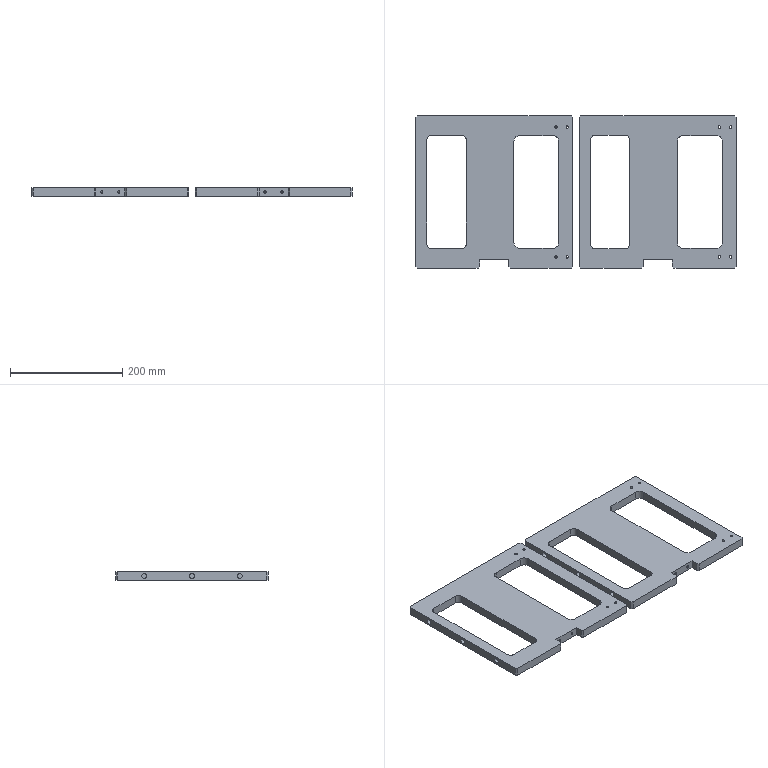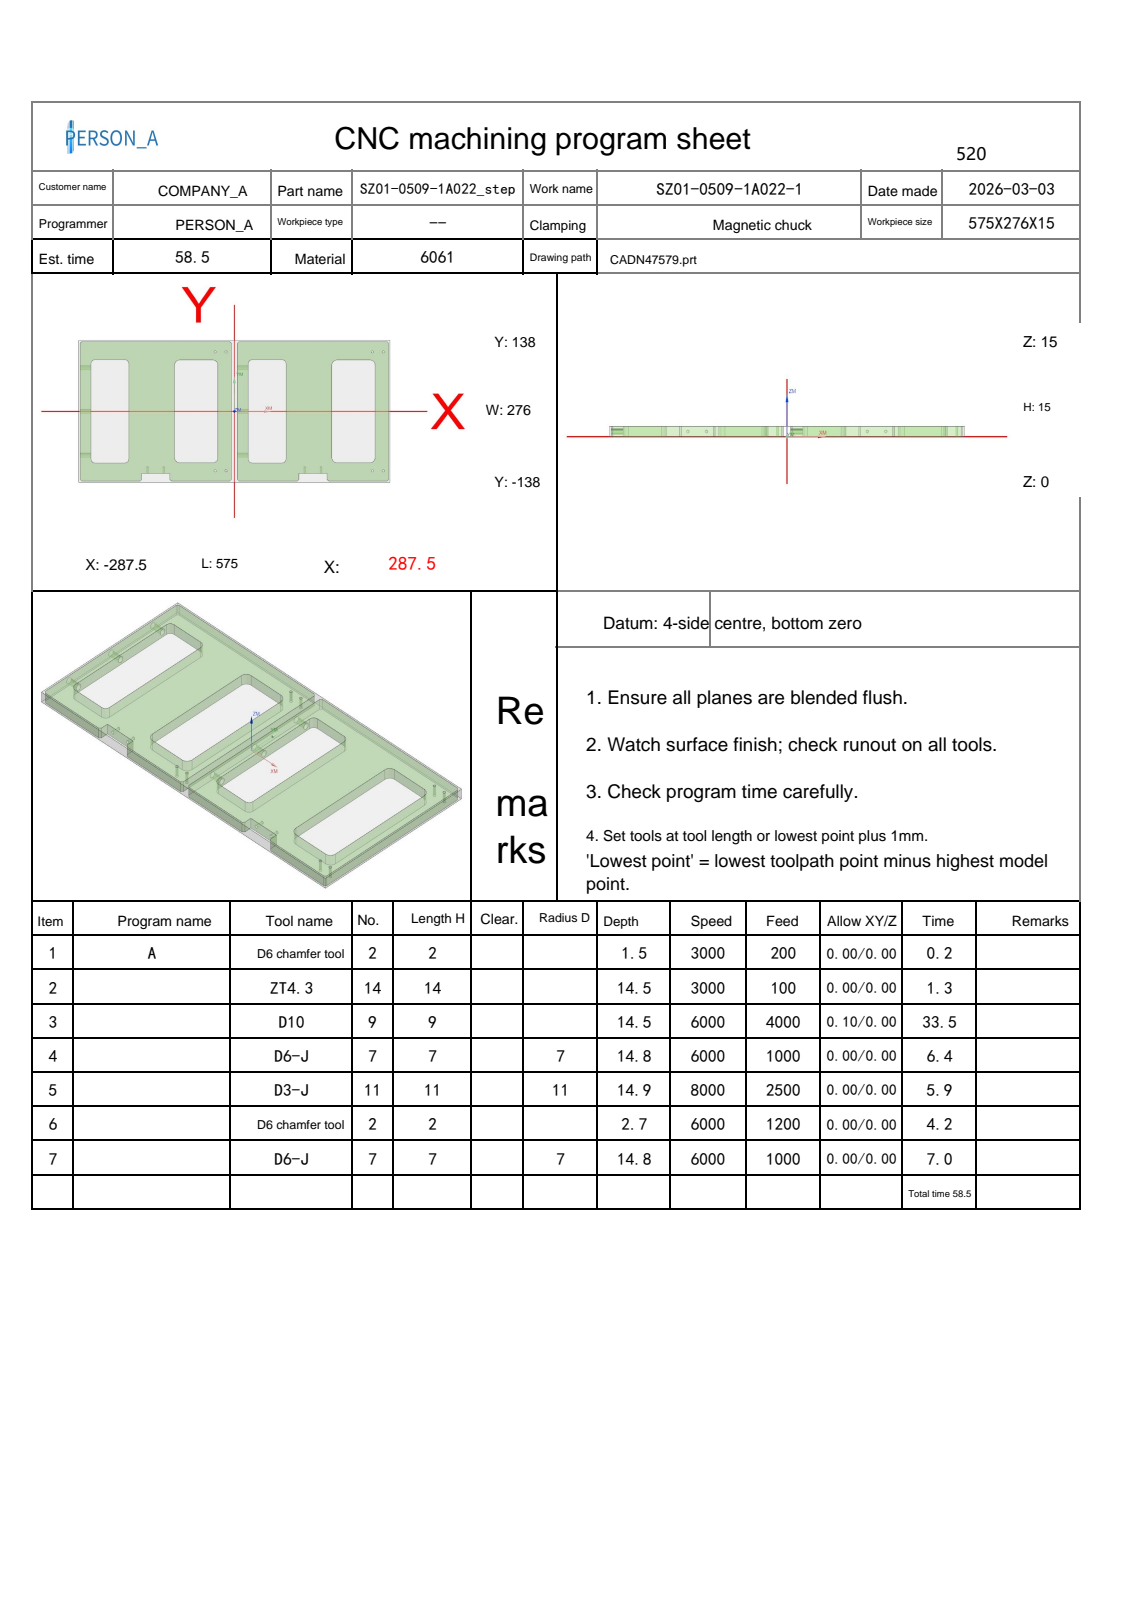NC program | NX | posted by the shop | part box 570 x 271 x 15 mm
Lines 57 to 971 of 10286:
N3 T09 M06
(D10  D=10. R=0. H=09 ce=0.10 di=0.00)
(MAX_Z=45. MIN_Z=0.5 Time=33.56M)
G00 G90 G54 X-35.6 Y0.0 M03 S6000
G43 H09 Z45.
M08
Z15.5
G01 Y90. Z15.412 F4000.
G03 X-40.5 Y94.9 Z15.404 I-4.9 J0.0
G01 X-100.5 Z15.346
G03 X-105.4 Y90. Z15.338 I0.0 J-4.9
G01 Y-90. Z15.162
G03 X-100.5 Y-94.9 Z15.154 I4.9 J0.0
G01 X-40.5 Z15.096
G03 X-35.6 Y-90. Z15.088 I0.0 J4.9
G01 Y90. Z14.912
G03 X-40.5 Y94.9 Z14.904 I-4.9 J0.0
G01 X-100.5 Z14.846
G03 X-105.4 Y90. Z14.838 I0.0 J-4.9
G01 Y-90. Z14.662
G03 X-100.5 Y-94.9 Z14.654 I4.9 J0.0
G01 X-40.5 Z14.596
G03 X-35.6 Y-90. Z14.588 I0.0 J4.9
G01 Y90. Z14.412
G03 X-40.5 Y94.9 Z14.404 I-4.9 J0.0
G01 X-100.5 Z14.346
G03 X-105.4 Y90. Z14.338 I0.0 J-4.9
G01 Y-90. Z14.162
G03 X-100.5 Y-94.9 Z14.154 I4.9 J0.0
G01 X-40.5 Z14.096
G03 X-35.6 Y-90. Z14.088 I0.0 J4.9
G01 Y90. Z13.912
G03 X-40.5 Y94.9 Z13.904 I-4.9 J0.0
G01 X-100.5 Z13.846
G03 X-105.4 Y90. Z13.838 I0.0 J-4.9
G01 Y-90. Z13.662
G03 X-100.5 Y-94.9 Z13.654 I4.9 J0.0
G01 X-40.5 Z13.596
G03 X-35.6 Y-90. Z13.588 I0.0 J4.9
G01 Y90. Z13.412
G03 X-40.5 Y94.9 Z13.404 I-4.9 J0.0
G01 X-100.5 Z13.346
G03 X-105.4 Y90. Z13.338 I0.0 J-4.9
G01 Y-90. Z13.162
G03 X-100.5 Y-94.9 Z13.154 I4.9 J0.0
G01 X-40.5 Z13.096
G03 X-35.6 Y-90. Z13.088 I0.0 J4.9
G01 Y90. Z12.912
G03 X-40.5 Y94.9 Z12.904 I-4.9 J0.0
G01 X-100.5 Z12.846
G03 X-105.4 Y90. Z12.838 I0.0 J-4.9
G01 Y-90. Z12.662
G03 X-100.5 Y-94.9 Z12.654 I4.9 J0.0
G01 X-40.5 Z12.596
G03 X-35.6 Y-90. Z12.588 I0.0 J4.9
G01 Y90. Z12.412
G03 X-40.5 Y94.9 Z12.404 I-4.9 J0.0
G01 X-100.5 Z12.346
G03 X-105.4 Y90. Z12.338 I0.0 J-4.9
G01 Y-90. Z12.162
G03 X-100.5 Y-94.9 Z12.154 I4.9 J0.0
G01 X-40.5 Z12.096
G03 X-35.6 Y-90. Z12.088 I0.0 J4.9
G01 Y90. Z11.912
G03 X-40.5 Y94.9 Z11.904 I-4.9 J0.0
G01 X-100.5 Z11.846
G03 X-105.4 Y90. Z11.838 I0.0 J-4.9
G01 Y-90. Z11.662
G03 X-100.5 Y-94.9 Z11.654 I4.9 J0.0
G01 X-40.5 Z11.596
G03 X-35.6 Y-90. Z11.588 I0.0 J4.9
G01 Y90. Z11.412
G03 X-40.5 Y94.9 Z11.404 I-4.9 J0.0
G01 X-100.5 Z11.346
G03 X-105.4 Y90. Z11.338 I0.0 J-4.9
G01 Y-90. Z11.162
G03 X-100.5 Y-94.9 Z11.154 I4.9 J0.0
G01 X-40.5 Z11.096
G03 X-35.6 Y-90. Z11.088 I0.0 J4.9
G01 Y90. Z10.912
G03 X-40.5 Y94.9 Z10.904 I-4.9 J0.0
G01 X-100.5 Z10.846
G03 X-105.4 Y90. Z10.838 I0.0 J-4.9
G01 Y-90. Z10.662
G03 X-100.5 Y-94.9 Z10.654 I4.9 J0.0
G01 X-40.5 Z10.596
G03 X-35.6 Y-90. Z10.588 I0.0 J4.9
G01 Y90. Z10.412
G03 X-40.5 Y94.9 Z10.404 I-4.9 J0.0
G01 X-100.5 Z10.346
G03 X-105.4 Y90. Z10.338 I0.0 J-4.9
G01 Y-90. Z10.162
G03 X-100.5 Y-94.9 Z10.154 I4.9 J0.0
G01 X-40.5 Z10.096
G03 X-35.6 Y-90. Z10.088 I0.0 J4.9
G01 Y90. Z9.912
G03 X-40.5 Y94.9 Z9.904 I-4.9 J0.0
G01 X-100.5 Z9.846
G03 X-105.4 Y90. Z9.838 I0.0 J-4.9
G01 Y-90. Z9.662
G03 X-100.5 Y-94.9 Z9.654 I4.9 J0.0
G01 X-40.5 Z9.596
G03 X-35.6 Y-90. Z9.588 I0.0 J4.9
G01 Y90. Z9.412
G03 X-40.5 Y94.9 Z9.404 I-4.9 J0.0
G01 X-100.5 Z9.346
G03 X-105.4 Y90. Z9.338 I0.0 J-4.9
G01 Y-90. Z9.162
G03 X-100.5 Y-94.9 Z9.154 I4.9 J0.0
G01 X-40.5 Z9.096
G03 X-35.6 Y-90. Z9.088 I0.0 J4.9
G01 Y90. Z8.912
G03 X-40.5 Y94.9 Z8.904 I-4.9 J0.0
G01 X-100.5 Z8.846
G03 X-105.4 Y90. Z8.838 I0.0 J-4.9
G01 Y-90. Z8.662
G03 X-100.5 Y-94.9 Z8.654 I4.9 J0.0
G01 X-40.5 Z8.596
G03 X-35.6 Y-90. Z8.588 I0.0 J4.9
G01 Y90. Z8.412
G03 X-40.5 Y94.9 Z8.404 I-4.9 J0.0
G01 X-100.5 Z8.346
G03 X-105.4 Y90. Z8.338 I0.0 J-4.9
G01 Y-90. Z8.162
G03 X-100.5 Y-94.9 Z8.154 I4.9 J0.0
G01 X-40.5 Z8.096
G03 X-35.6 Y-90. Z8.088 I0.0 J4.9
G01 Y90. Z7.912
G03 X-40.5 Y94.9 Z7.904 I-4.9 J0.0
G01 X-100.5 Z7.846
G03 X-105.4 Y90. Z7.838 I0.0 J-4.9
G01 Y-90. Z7.662
G03 X-100.5 Y-94.9 Z7.654 I4.9 J0.0
G01 X-40.5 Z7.596
G03 X-35.6 Y-90. Z7.588 I0.0 J4.9
G01 Y90. Z7.412
G03 X-40.5 Y94.9 Z7.404 I-4.9 J0.0
G01 X-100.5 Z7.346
G03 X-105.4 Y90. Z7.338 I0.0 J-4.9
G01 Y-90. Z7.162
G03 X-100.5 Y-94.9 Z7.154 I4.9 J0.0
G01 X-40.5 Z7.096
G03 X-35.6 Y-90. Z7.088 I0.0 J4.9
G01 Y90. Z6.912
G03 X-40.5 Y94.9 Z6.904 I-4.9 J0.0
G01 X-100.5 Z6.846
G03 X-105.4 Y90. Z6.838 I0.0 J-4.9
G01 Y-90. Z6.662
G03 X-100.5 Y-94.9 Z6.654 I4.9 J0.0
G01 X-40.5 Z6.596
G03 X-35.6 Y-90. Z6.588 I0.0 J4.9
G01 Y90. Z6.412
G03 X-40.5 Y94.9 Z6.404 I-4.9 J0.0
G01 X-100.5 Z6.346
G03 X-105.4 Y90. Z6.338 I0.0 J-4.9
G01 Y-90. Z6.162
G03 X-100.5 Y-94.9 Z6.154 I4.9 J0.0
G01 X-40.5 Z6.096
G03 X-35.6 Y-90. Z6.088 I0.0 J4.9
G01 Y90. Z5.912
G03 X-40.5 Y94.9 Z5.904 I-4.9 J0.0
G01 X-100.5 Z5.846
G03 X-105.4 Y90. Z5.838 I0.0 J-4.9
G01 Y-90. Z5.662
G03 X-100.5 Y-94.9 Z5.654 I4.9 J0.0
G01 X-40.5 Z5.596
G03 X-35.6 Y-90. Z5.588 I0.0 J4.9
G01 Y90. Z5.412
G03 X-40.5 Y94.9 Z5.404 I-4.9 J0.0
G01 X-100.5 Z5.346
G03 X-105.4 Y90. Z5.338 I0.0 J-4.9
G01 Y-90. Z5.162
G03 X-100.5 Y-94.9 Z5.154 I4.9 J0.0
G01 X-40.5 Z5.096
G03 X-35.6 Y-90. Z5.088 I0.0 J4.9
G01 Y90. Z4.912
G03 X-40.5 Y94.9 Z4.904 I-4.9 J0.0
G01 X-100.5 Z4.846
G03 X-105.4 Y90. Z4.838 I0.0 J-4.9
G01 Y-90. Z4.662
G03 X-100.5 Y-94.9 Z4.654 I4.9 J0.0
G01 X-40.5 Z4.596
G03 X-35.6 Y-90. Z4.588 I0.0 J4.9
G01 Y90. Z4.412
G03 X-40.5 Y94.9 Z4.404 I-4.9 J0.0
G01 X-100.5 Z4.346
G03 X-105.4 Y90. Z4.338 I0.0 J-4.9
G01 Y-90. Z4.162
G03 X-100.5 Y-94.9 Z4.154 I4.9 J0.0
G01 X-40.5 Z4.096
G03 X-35.6 Y-90. Z4.088 I0.0 J4.9
G01 Y90. Z3.912
G03 X-40.5 Y94.9 Z3.904 I-4.9 J0.0
G01 X-100.5 Z3.846
G03 X-105.4 Y90. Z3.838 I0.0 J-4.9
G01 Y-90. Z3.662
G03 X-100.5 Y-94.9 Z3.654 I4.9 J0.0
G01 X-40.5 Z3.596
G03 X-35.6 Y-90. Z3.588 I0.0 J4.9
G01 Y90. Z3.412
G03 X-40.5 Y94.9 Z3.404 I-4.9 J0.0
G01 X-100.5 Z3.346
G03 X-105.4 Y90. Z3.338 I0.0 J-4.9
G01 Y-90. Z3.162
G03 X-100.5 Y-94.9 Z3.154 I4.9 J0.0
G01 X-40.5 Z3.096
G03 X-35.6 Y-90. Z3.088 I0.0 J4.9
G01 Y90. Z2.912
G03 X-40.5 Y94.9 Z2.904 I-4.9 J0.0
G01 X-100.5 Z2.846
G03 X-105.4 Y90. Z2.838 I0.0 J-4.9
G01 Y-90. Z2.662
G03 X-100.5 Y-94.9 Z2.654 I4.9 J0.0
G01 X-40.5 Z2.596
G03 X-35.6 Y-90. Z2.588 I0.0 J4.9
G01 Y90. Z2.412
G03 X-40.5 Y94.9 Z2.404 I-4.9 J0.0
G01 X-100.5 Z2.346
G03 X-105.4 Y90. Z2.338 I0.0 J-4.9
G01 Y-90. Z2.162
G03 X-100.5 Y-94.9 Z2.154 I4.9 J0.0
G01 X-40.5 Z2.096
G03 X-35.6 Y-90. Z2.088 I0.0 J4.9
G01 Y90. Z1.912
G03 X-40.5 Y94.9 Z1.904 I-4.9 J0.0
G01 X-100.5 Z1.846
G03 X-105.4 Y90. Z1.838 I0.0 J-4.9
G01 Y-90. Z1.662
G03 X-100.5 Y-94.9 Z1.654 I4.9 J0.0
G01 X-40.5 Z1.596
G03 X-35.6 Y-90. Z1.588 I0.0 J4.9
G01 Y90. Z1.412
G03 X-40.5 Y94.9 Z1.404 I-4.9 J0.0
G01 X-100.5 Z1.346
G03 X-105.4 Y90. Z1.338 I0.0 J-4.9
G01 Y-90. Z1.162
G03 X-100.5 Y-94.9 Z1.154 I4.9 J0.0
G01 X-40.5 Z1.096
G03 X-35.6 Y-90. Z1.088 I0.0 J4.9
G01 Y90. Z.912
G03 X-40.5 Y94.9 Z.904 I-4.9 J0.0
G01 X-100.5 Z.846
G03 X-105.4 Y90. Z.838 I0.0 J-4.9
G01 Y-90. Z.662
G03 X-100.5 Y-94.9 Z.654 I4.9 J0.0
G01 X-40.5 Z.596
G03 X-35.6 Y-90. Z.588 I0.0 J4.9
G01 Y0.0 Z.5
Y90.
G03 X-40.5 Y94.9 I-4.9 J0.0
G01 X-100.5
G03 X-105.4 Y90. I0.0 J-4.9
G01 Y-90.
G03 X-100.5 Y-94.9 I4.9 J0.0
G01 X-40.5
G03 X-35.6 Y-90. I0.0 J4.9
G01 Y0.0
Y.5
Z1.5
G00 Z45.
X254.9 Y0.0
Z15.5
G01 Y90. Z15.412
G03 X251.612 Y94.627 Z15.406 I-4.9 J0.0
X250. Y94.9 Z15.404 I-1.612 J-4.627
G01 X190. Z15.346
G03 X185.1 Y90. Z15.338 I0.0 J-4.9
G01 Y-90. Z15.162
G03 X190. Y-94.9 Z15.154 I4.9 J0.0
G01 X250. Z15.096
G03 X254.9 Y-90. Z15.088 I0.0 J4.9
G01 Y90. Z14.912
G03 X251.612 Y94.627 Z14.906 I-4.9 J0.0
X250. Y94.9 Z14.904 I-1.612 J-4.627
G01 X190. Z14.846
G03 X185.1 Y90. Z14.838 I0.0 J-4.9
G01 Y-90. Z14.662
G03 X190. Y-94.9 Z14.654 I4.9 J0.0
G01 X250. Z14.596
G03 X254.9 Y-90. Z14.588 I0.0 J4.9
G01 Y90. Z14.412
G03 X251.612 Y94.627 Z14.406 I-4.9 J0.0
X250. Y94.9 Z14.404 I-1.612 J-4.627
G01 X190. Z14.346
G03 X185.1 Y90. Z14.338 I0.0 J-4.9
G01 Y-90. Z14.162
G03 X190. Y-94.9 Z14.154 I4.9 J0.0
G01 X250. Z14.096
G03 X254.9 Y-90. Z14.088 I0.0 J4.9
G01 Y90. Z13.912
G03 X251.612 Y94.627 Z13.906 I-4.9 J0.0
X250. Y94.9 Z13.904 I-1.612 J-4.627
G01 X190. Z13.846
G03 X185.1 Y90. Z13.838 I0.0 J-4.9
G01 Y-90. Z13.662
G03 X190. Y-94.9 Z13.654 I4.9 J0.0
G01 X250. Z13.596
G03 X254.9 Y-90. Z13.588 I0.0 J4.9
G01 Y90. Z13.412
G03 X251.612 Y94.627 Z13.406 I-4.9 J0.0
X250. Y94.9 Z13.404 I-1.612 J-4.627
G01 X190. Z13.346
G03 X185.1 Y90. Z13.338 I0.0 J-4.9
G01 Y-90. Z13.162
G03 X190. Y-94.9 Z13.154 I4.9 J0.0
G01 X250. Z13.096
G03 X254.9 Y-90. Z13.088 I0.0 J4.9
G01 Y90. Z12.912
G03 X251.612 Y94.627 Z12.906 I-4.9 J0.0
X250. Y94.9 Z12.904 I-1.612 J-4.627
G01 X190. Z12.846
G03 X185.1 Y90. Z12.838 I0.0 J-4.9
G01 Y-90. Z12.662
G03 X190. Y-94.9 Z12.654 I4.9 J0.0
G01 X250. Z12.596
G03 X254.9 Y-90. Z12.588 I0.0 J4.9
G01 Y90. Z12.412
G03 X251.612 Y94.627 Z12.406 I-4.9 J0.0
X250. Y94.9 Z12.404 I-1.612 J-4.627
G01 X190. Z12.346
G03 X185.1 Y90. Z12.338 I0.0 J-4.9
G01 Y-90. Z12.162
G03 X190. Y-94.9 Z12.154 I4.9 J0.0
G01 X250. Z12.096
G03 X254.9 Y-90. Z12.088 I0.0 J4.9
G01 Y90. Z11.912
G03 X251.612 Y94.627 Z11.906 I-4.9 J0.0
X250. Y94.9 Z11.904 I-1.612 J-4.627
G01 X190. Z11.846
G03 X185.1 Y90. Z11.838 I0.0 J-4.9
G01 Y-90. Z11.662
G03 X190. Y-94.9 Z11.654 I4.9 J0.0
G01 X250. Z11.596
G03 X254.9 Y-90. Z11.588 I0.0 J4.9
G01 Y90. Z11.412
G03 X251.612 Y94.627 Z11.406 I-4.9 J0.0
X250. Y94.9 Z11.404 I-1.612 J-4.627
G01 X190. Z11.346
G03 X185.1 Y90. Z11.338 I0.0 J-4.9
G01 Y-90. Z11.162
G03 X190. Y-94.9 Z11.154 I4.9 J0.0
G01 X250. Z11.096
G03 X254.9 Y-90. Z11.088 I0.0 J4.9
G01 Y90. Z10.912
G03 X251.612 Y94.627 Z10.906 I-4.9 J0.0
X250. Y94.9 Z10.904 I-1.612 J-4.627
G01 X190. Z10.846
G03 X185.1 Y90. Z10.838 I0.0 J-4.9
G01 Y-90. Z10.662
G03 X190. Y-94.9 Z10.654 I4.9 J0.0
G01 X250. Z10.596
G03 X254.9 Y-90. Z10.588 I0.0 J4.9
G01 Y90. Z10.412
G03 X251.612 Y94.627 Z10.406 I-4.9 J0.0
X250. Y94.9 Z10.404 I-1.612 J-4.627
G01 X190. Z10.346
G03 X185.1 Y90. Z10.338 I0.0 J-4.9
G01 Y-90. Z10.162
G03 X190. Y-94.9 Z10.154 I4.9 J0.0
G01 X250. Z10.096
G03 X254.9 Y-90. Z10.088 I0.0 J4.9
G01 Y90. Z9.912
G03 X251.612 Y94.627 Z9.906 I-4.9 J0.0
X250. Y94.9 Z9.904 I-1.612 J-4.627
G01 X190. Z9.846
G03 X185.1 Y90. Z9.838 I0.0 J-4.9
G01 Y-90. Z9.662
G03 X190. Y-94.9 Z9.654 I4.9 J0.0
G01 X250. Z9.596
G03 X254.9 Y-90. Z9.588 I0.0 J4.9
G01 Y90. Z9.412
G03 X251.612 Y94.627 Z9.406 I-4.9 J0.0
X250. Y94.9 Z9.404 I-1.612 J-4.627
G01 X190. Z9.346
G03 X185.1 Y90. Z9.338 I0.0 J-4.9
G01 Y-90. Z9.162
G03 X190. Y-94.9 Z9.154 I4.9 J0.0
G01 X250. Z9.096
G03 X254.9 Y-90. Z9.088 I0.0 J4.9
G01 Y90. Z8.912
G03 X251.612 Y94.627 Z8.906 I-4.9 J0.0
X250. Y94.9 Z8.904 I-1.612 J-4.627
G01 X190. Z8.846
G03 X185.1 Y90. Z8.838 I0.0 J-4.9
G01 Y-90. Z8.662
G03 X190. Y-94.9 Z8.654 I4.9 J0.0
G01 X250. Z8.596
G03 X254.9 Y-90. Z8.588 I0.0 J4.9
G01 Y90. Z8.412
G03 X251.612 Y94.627 Z8.406 I-4.9 J0.0
X250. Y94.9 Z8.404 I-1.612 J-4.627
G01 X190. Z8.346
G03 X185.1 Y90. Z8.338 I0.0 J-4.9
G01 Y-90. Z8.162
G03 X190. Y-94.9 Z8.154 I4.9 J0.0
G01 X250. Z8.096
G03 X254.9 Y-90. Z8.088 I0.0 J4.9
G01 Y90. Z7.912
G03 X251.612 Y94.627 Z7.906 I-4.9 J0.0
X250. Y94.9 Z7.904 I-1.612 J-4.627
G01 X190. Z7.846
G03 X185.1 Y90. Z7.838 I0.0 J-4.9
G01 Y-90. Z7.662
G03 X190. Y-94.9 Z7.654 I4.9 J0.0
G01 X250. Z7.596
G03 X254.9 Y-90. Z7.588 I0.0 J4.9
G01 Y90. Z7.412
G03 X251.612 Y94.627 Z7.406 I-4.9 J0.0
X250. Y94.9 Z7.404 I-1.612 J-4.627
G01 X190. Z7.346
G03 X185.1 Y90. Z7.338 I0.0 J-4.9
G01 Y-90. Z7.162
G03 X190. Y-94.9 Z7.154 I4.9 J0.0
G01 X250. Z7.096
G03 X254.9 Y-90. Z7.088 I0.0 J4.9
G01 Y90. Z6.912
G03 X251.612 Y94.627 Z6.906 I-4.9 J0.0
X250. Y94.9 Z6.904 I-1.612 J-4.627
G01 X190. Z6.846
G03 X185.1 Y90. Z6.838 I0.0 J-4.9
G01 Y-90. Z6.662
G03 X190. Y-94.9 Z6.654 I4.9 J0.0
G01 X250. Z6.596
G03 X254.9 Y-90. Z6.588 I0.0 J4.9
G01 Y90. Z6.412
G03 X251.612 Y94.627 Z6.406 I-4.9 J0.0
X250. Y94.9 Z6.404 I-1.612 J-4.627
G01 X190. Z6.346
G03 X185.1 Y90. Z6.338 I0.0 J-4.9
G01 Y-90. Z6.162
G03 X190. Y-94.9 Z6.154 I4.9 J0.0
G01 X250. Z6.096
G03 X254.9 Y-90. Z6.088 I0.0 J4.9
G01 Y90. Z5.912
G03 X251.612 Y94.627 Z5.906 I-4.9 J0.0
X250. Y94.9 Z5.904 I-1.612 J-4.627
G01 X190. Z5.846
G03 X185.1 Y90. Z5.838 I0.0 J-4.9
G01 Y-90. Z5.662
G03 X190. Y-94.9 Z5.654 I4.9 J0.0
G01 X250. Z5.596
G03 X254.9 Y-90. Z5.588 I0.0 J4.9
G01 Y90. Z5.412
G03 X251.612 Y94.627 Z5.406 I-4.9 J0.0
X250. Y94.9 Z5.404 I-1.612 J-4.627
G01 X190. Z5.346
G03 X185.1 Y90. Z5.338 I0.0 J-4.9
G01 Y-90. Z5.162
G03 X190. Y-94.9 Z5.154 I4.9 J0.0
G01 X250. Z5.096
G03 X254.9 Y-90. Z5.088 I0.0 J4.9
G01 Y90. Z4.912
G03 X251.612 Y94.627 Z4.906 I-4.9 J0.0
X250. Y94.9 Z4.904 I-1.612 J-4.627
G01 X190. Z4.846
G03 X185.1 Y90. Z4.838 I0.0 J-4.9
G01 Y-90. Z4.662
G03 X190. Y-94.9 Z4.654 I4.9 J0.0
G01 X250. Z4.596
G03 X254.9 Y-90. Z4.588 I0.0 J4.9
G01 Y90. Z4.412
G03 X251.612 Y94.627 Z4.406 I-4.9 J0.0
X250. Y94.9 Z4.404 I-1.612 J-4.627
G01 X190. Z4.346
G03 X185.1 Y90. Z4.338 I0.0 J-4.9
G01 Y-90. Z4.162
G03 X190. Y-94.9 Z4.154 I4.9 J0.0
G01 X250. Z4.096
G03 X254.9 Y-90. Z4.088 I0.0 J4.9
G01 Y90. Z3.912
G03 X251.612 Y94.627 Z3.906 I-4.9 J0.0
X250. Y94.9 Z3.904 I-1.612 J-4.627
G01 X190. Z3.846
G03 X185.1 Y90. Z3.838 I0.0 J-4.9
G01 Y-90. Z3.662
G03 X190. Y-94.9 Z3.654 I4.9 J0.0
G01 X250. Z3.596
G03 X254.9 Y-90. Z3.588 I0.0 J4.9
G01 Y90. Z3.412
G03 X251.612 Y94.627 Z3.406 I-4.9 J0.0
X250. Y94.9 Z3.404 I-1.612 J-4.627
G01 X190. Z3.346
G03 X185.1 Y90. Z3.338 I0.0 J-4.9
G01 Y-90. Z3.162
G03 X190. Y-94.9 Z3.154 I4.9 J0.0
G01 X250. Z3.096
G03 X254.9 Y-90. Z3.088 I0.0 J4.9
G01 Y90. Z2.912
G03 X251.612 Y94.627 Z2.906 I-4.9 J0.0
X250. Y94.9 Z2.904 I-1.612 J-4.627
G01 X190. Z2.846
G03 X185.1 Y90. Z2.838 I0.0 J-4.9
G01 Y-90. Z2.662
G03 X190. Y-94.9 Z2.654 I4.9 J0.0
G01 X250. Z2.596
G03 X254.9 Y-90. Z2.588 I0.0 J4.9
G01 Y90. Z2.412
G03 X251.612 Y94.627 Z2.406 I-4.9 J0.0
X250. Y94.9 Z2.404 I-1.612 J-4.627
G01 X190. Z2.346
G03 X185.1 Y90. Z2.338 I0.0 J-4.9
G01 Y-90. Z2.162
G03 X190. Y-94.9 Z2.154 I4.9 J0.0
G01 X250. Z2.096
G03 X254.9 Y-90. Z2.088 I0.0 J4.9
G01 Y90. Z1.912
G03 X251.612 Y94.627 Z1.906 I-4.9 J0.0
X250. Y94.9 Z1.904 I-1.612 J-4.627
G01 X190. Z1.846
G03 X185.1 Y90. Z1.838 I0.0 J-4.9
G01 Y-90. Z1.662
G03 X190. Y-94.9 Z1.654 I4.9 J0.0
G01 X250. Z1.596
G03 X254.9 Y-90. Z1.588 I0.0 J4.9
G01 Y90. Z1.412
G03 X251.612 Y94.627 Z1.406 I-4.9 J0.0
X250. Y94.9 Z1.404 I-1.612 J-4.627
G01 X190. Z1.346
G03 X185.1 Y90. Z1.338 I0.0 J-4.9
G01 Y-90. Z1.162
G03 X190. Y-94.9 Z1.154 I4.9 J0.0
G01 X250. Z1.096
G03 X254.9 Y-90. Z1.088 I0.0 J4.9
G01 Y90. Z.912
G03 X251.612 Y94.627 Z.906 I-4.9 J0.0
X250. Y94.9 Z.904 I-1.612 J-4.627
G01 X190. Z.846
G03 X185.1 Y90. Z.838 I0.0 J-4.9
G01 Y-90. Z.662
G03 X190. Y-94.9 Z.654 I4.9 J0.0
G01 X250. Z.596
G03 X254.9 Y-90. Z.588 I0.0 J4.9
G01 Y0.0 Z.5
Y90.
G03 X250. Y94.9 I-4.9 J0.0
G01 X190.
G03 X185.1 Y90. I0.0 J-4.9
G01 Y-90.
G03 X190. Y-94.9 I4.9 J0.0
G01 X250.
G03 X254.9 Y-90. I0.0 J4.9
G01 Y0.0
Y.5
Z1.5
G00 Z45.
G00 G90 X-259.9 Y0.0 M03 S6000
Z45.
Z15.5
G01 Y-92.5 Z15.407 F4000.
G03 X-257. Y-95.4 Z15.402 I2.9 J0.0
G01 X-203. Z15.348
G03 X-200.1 Y-92.5 Z15.343 I0.0 J2.9
G01 Y92.5 Z15.157
G03 X-203. Y95.4 Z15.152 I-2.9 J0.0
G01 X-257. Z15.098
G03 X-259.9 Y92.5 Z15.093 I0.0 J-2.9
G01 Y-92.5 Z14.907
G03 X-257. Y-95.4 Z14.902 I2.9 J0.0
G01 X-203. Z14.848
G03 X-200.1 Y-92.5 Z14.843 I0.0 J2.9
G01 Y92.5 Z14.657
G03 X-203. Y95.4 Z14.652 I-2.9 J0.0
G01 X-257. Z14.598
G03 X-259.9 Y92.5 Z14.593 I0.0 J-2.9
G01 Y-92.5 Z14.407
G03 X-257. Y-95.4 Z14.402 I2.9 J0.0
G01 X-203. Z14.348
G03 X-200.1 Y-92.5 Z14.343 I0.0 J2.9
G01 Y92.5 Z14.157
G03 X-203. Y95.4 Z14.152 I-2.9 J0.0
G01 X-257. Z14.098
G03 X-259.9 Y92.5 Z14.093 I0.0 J-2.9
G01 Y-92.5 Z13.907
G03 X-257. Y-95.4 Z13.902 I2.9 J0.0
G01 X-203. Z13.848
G03 X-200.1 Y-92.5 Z13.843 I0.0 J2.9
G01 Y92.5 Z13.657
G03 X-203. Y95.4 Z13.652 I-2.9 J0.0
G01 X-257. Z13.598
G03 X-259.9 Y92.5 Z13.593 I0.0 J-2.9
G01 Y-92.5 Z13.407
G03 X-257. Y-95.4 Z13.402 I2.9 J0.0
G01 X-203. Z13.348
G03 X-200.1 Y-92.5 Z13.343 I0.0 J2.9
G01 Y92.5 Z13.157
G03 X-203. Y95.4 Z13.152 I-2.9 J0.0
G01 X-257. Z13.098
G03 X-259.9 Y92.5 Z13.093 I0.0 J-2.9
G01 Y-92.5 Z12.907
G03 X-257. Y-95.4 Z12.902 I2.9 J0.0
G01 X-203. Z12.848
G03 X-200.1 Y-92.5 Z12.843 I0.0 J2.9
G01 Y92.5 Z12.657
G03 X-203. Y95.4 Z12.652 I-2.9 J0.0
G01 X-257. Z12.598
G03 X-259.9 Y92.5 Z12.593 I0.0 J-2.9
G01 Y-92.5 Z12.407
G03 X-257. Y-95.4 Z12.402 I2.9 J0.0
G01 X-203. Z12.348
G03 X-200.1 Y-92.5 Z12.343 I0.0 J2.9
G01 Y92.5 Z12.157
G03 X-203. Y95.4 Z12.152 I-2.9 J0.0
G01 X-257. Z12.098
G03 X-259.9 Y92.5 Z12.093 I0.0 J-2.9
G01 Y-92.5 Z11.907
G03 X-257. Y-95.4 Z11.902 I2.9 J0.0
G01 X-203. Z11.848
G03 X-200.1 Y-92.5 Z11.843 I0.0 J2.9
G01 Y92.5 Z11.657
G03 X-203. Y95.4 Z11.652 I-2.9 J0.0
G01 X-257. Z11.598
G03 X-259.9 Y92.5 Z11.593 I0.0 J-2.9
G01 Y-92.5 Z11.407
G03 X-257. Y-95.4 Z11.402 I2.9 J0.0
G01 X-203. Z11.348
G03 X-200.1 Y-92.5 Z11.343 I0.0 J2.9
G01 Y92.5 Z11.157
G03 X-203. Y95.4 Z11.152 I-2.9 J0.0
G01 X-257. Z11.098
G03 X-259.9 Y92.5 Z11.093 I0.0 J-2.9
G01 Y-92.5 Z10.907
G03 X-257. Y-95.4 Z10.902 I2.9 J0.0
G01 X-203. Z10.848
G03 X-200.1 Y-92.5 Z10.843 I0.0 J2.9
G01 Y92.5 Z10.657
G03 X-203. Y95.4 Z10.652 I-2.9 J0.0
G01 X-257. Z10.598
G03 X-259.9 Y92.5 Z10.593 I0.0 J-2.9
G01 Y-92.5 Z10.407
G03 X-257. Y-95.4 Z10.402 I2.9 J0.0
G01 X-203. Z10.348
G03 X-200.1 Y-92.5 Z10.343 I0.0 J2.9
G01 Y92.5 Z10.157
G03 X-203. Y95.4 Z10.152 I-2.9 J0.0
G01 X-257. Z10.098
G03 X-259.9 Y92.5 Z10.093 I0.0 J-2.9
G01 Y-92.5 Z9.907
G03 X-257. Y-95.4 Z9.902 I2.9 J0.0
G01 X-203. Z9.848
G03 X-200.1 Y-92.5 Z9.843 I0.0 J2.9
G01 Y92.5 Z9.657
G03 X-203. Y95.4 Z9.652 I-2.9 J0.0
G01 X-257. Z9.598
G03 X-259.9 Y92.5 Z9.593 I0.0 J-2.9
G01 Y-92.5 Z9.407
G03 X-257. Y-95.4 Z9.402 I2.9 J0.0
G01 X-203. Z9.348
G03 X-200.1 Y-92.5 Z9.343 I0.0 J2.9
G01 Y92.5 Z9.157
G03 X-203. Y95.4 Z9.152 I-2.9 J0.0
G01 X-257. Z9.098
G03 X-259.9 Y92.5 Z9.093 I0.0 J-2.9
G01 Y-92.5 Z8.907
G03 X-257. Y-95.4 Z8.902 I2.9 J0.0
G01 X-203. Z8.848
G03 X-200.1 Y-92.5 Z8.843 I0.0 J2.9
G01 Y92.5 Z8.657
G03 X-203. Y95.4 Z8.652 I-2.9 J0.0
G01 X-257. Z8.598
G03 X-259.9 Y92.5 Z8.593 I0.0 J-2.9
G01 Y-92.5 Z8.407
G03 X-257. Y-95.4 Z8.402 I2.9 J0.0
G01 X-203. Z8.348
G03 X-200.1 Y-92.5 Z8.343 I0.0 J2.9
G01 Y92.5 Z8.157
G03 X-203. Y95.4 Z8.152 I-2.9 J0.0
G01 X-257. Z8.098
G03 X-259.9 Y92.5 Z8.093 I0.0 J-2.9
G01 Y-92.5 Z7.907
G03 X-257. Y-95.4 Z7.902 I2.9 J0.0
G01 X-203. Z7.848
G03 X-200.1 Y-92.5 Z7.843 I0.0 J2.9
G01 Y92.5 Z7.657
G03 X-203. Y95.4 Z7.652 I-2.9 J0.0
G01 X-257. Z7.598
G03 X-259.9 Y92.5 Z7.593 I0.0 J-2.9
G01 Y-92.5 Z7.407
G03 X-257. Y-95.4 Z7.402 I2.9 J0.0
G01 X-203. Z7.348
G03 X-200.1 Y-92.5 Z7.343 I0.0 J2.9
G01 Y92.5 Z7.157
G03 X-203. Y95.4 Z7.152 I-2.9 J0.0
G01 X-257. Z7.098
G03 X-259.9 Y92.5 Z7.093 I0.0 J-2.9
G01 Y-92.5 Z6.907
G03 X-257. Y-95.4 Z6.902 I2.9 J0.0
G01 X-203. Z6.848
G03 X-200.1 Y-92.5 Z6.843 I0.0 J2.9
G01 Y92.5 Z6.657
G03 X-203. Y95.4 Z6.652 I-2.9 J0.0
G01 X-257. Z6.598
G03 X-259.9 Y92.5 Z6.593 I0.0 J-2.9
G01 Y-92.5 Z6.407
G03 X-257. Y-95.4 Z6.402 I2.9 J0.0
G01 X-203. Z6.348
G03 X-200.1 Y-92.5 Z6.343 I0.0 J2.9
G01 Y92.5 Z6.157
G03 X-203. Y95.4 Z6.152 I-2.9 J0.0
G01 X-257. Z6.098
G03 X-259.9 Y92.5 Z6.093 I0.0 J-2.9
G01 Y-92.5 Z5.907
G03 X-257. Y-95.4 Z5.902 I2.9 J0.0
G01 X-203. Z5.848
G03 X-200.1 Y-92.5 Z5.843 I0.0 J2.9
G01 Y92.5 Z5.657
G03 X-203. Y95.4 Z5.652 I-2.9 J0.0
G01 X-257. Z5.598
G03 X-259.9 Y92.5 Z5.593 I0.0 J-2.9
G01 Y-92.5 Z5.407
G03 X-257. Y-95.4 Z5.402 I2.9 J0.0
G01 X-203. Z5.348
G03 X-200.1 Y-92.5 Z5.343 I0.0 J2.9
G01 Y92.5 Z5.157
G03 X-203. Y95.4 Z5.152 I-2.9 J0.0
G01 X-257. Z5.098
G03 X-259.9 Y92.5 Z5.093 I0.0 J-2.9
G01 Y-92.5 Z4.907
G03 X-257. Y-95.4 Z4.902 I2.9 J0.0
G01 X-203. Z4.848
G03 X-200.1 Y-92.5 Z4.843 I0.0 J2.9
G01 Y92.5 Z4.657
G03 X-203. Y95.4 Z4.652 I-2.9 J0.0
G01 X-257. Z4.598
G03 X-259.9 Y92.5 Z4.593 I0.0 J-2.9
G01 Y-92.5 Z4.407
G03 X-257. Y-95.4 Z4.402 I2.9 J0.0
G01 X-203. Z4.348
G03 X-200.1 Y-92.5 Z4.343 I0.0 J2.9
G01 Y92.5 Z4.157
G03 X-203. Y95.4 Z4.152 I-2.9 J0.0
G01 X-257. Z4.098
G03 X-259.9 Y92.5 Z4.093 I0.0 J-2.9
G01 Y-92.5 Z3.907
G03 X-257. Y-95.4 Z3.902 I2.9 J0.0
G01 X-203. Z3.848
G03 X-200.1 Y-92.5 Z3.843 I0.0 J2.9
G01 Y92.5 Z3.657
G03 X-203. Y95.4 Z3.652 I-2.9 J0.0
G01 X-257. Z3.598
G03 X-259.9 Y92.5 Z3.593 I0.0 J-2.9
G01 Y-92.5 Z3.407
G03 X-257. Y-95.4 Z3.402 I2.9 J0.0
G01 X-203. Z3.348
G03 X-200.1 Y-92.5 Z3.343 I0.0 J2.9
G01 Y92.5 Z3.157
G03 X-203. Y95.4 Z3.152 I-2.9 J0.0
G01 X-257. Z3.098
G03 X-259.9 Y92.5 Z3.093 I0.0 J-2.9
G01 Y-92.5 Z2.907
G03 X-257. Y-95.4 Z2.902 I2.9 J0.0
G01 X-203. Z2.848
G03 X-200.1 Y-92.5 Z2.843 I0.0 J2.9
G01 Y92.5 Z2.657
G03 X-203. Y95.4 Z2.652 I-2.9 J0.0
G01 X-257. Z2.598
G03 X-259.9 Y92.5 Z2.593 I0.0 J-2.9
G01 Y-92.5 Z2.407
G03 X-257. Y-95.4 Z2.402 I2.9 J0.0
G01 X-203. Z2.348
G03 X-200.1 Y-92.5 Z2.343 I0.0 J2.9
G01 Y92.5 Z2.157
G03 X-203. Y95.4 Z2.152 I-2.9 J0.0
G01 X-257. Z2.098
G03 X-259.9 Y92.5 Z2.093 I0.0 J-2.9
G01 Y-92.5 Z1.907
G03 X-257. Y-95.4 Z1.902 I2.9 J0.0
G01 X-203. Z1.848
G03 X-200.1 Y-92.5 Z1.843 I0.0 J2.9
G01 Y92.5 Z1.657
G03 X-203. Y95.4 Z1.652 I-2.9 J0.0
G01 X-257. Z1.598
G03 X-259.9 Y92.5 Z1.593 I0.0 J-2.9
G01 Y-92.5 Z1.407
G03 X-257. Y-95.4 Z1.402 I2.9 J0.0
G01 X-203. Z1.348
G03 X-200.1 Y-92.5 Z1.343 I0.0 J2.9
G01 Y92.5 Z1.157
G03 X-203. Y95.4 Z1.152 I-2.9 J0.0
G01 X-257. Z1.098
G03 X-259.9 Y92.5 Z1.093 I0.0 J-2.9
G01 Y-92.5 Z.907
G03 X-257. Y-95.4 Z.902 I2.9 J0.0
G01 X-203. Z.848
G03 X-200.1 Y-92.5 Z.843 I0.0 J2.9
G01 Y92.5 Z.657
G03 X-203. Y95.4 Z.652 I-2.9 J0.0
G01 X-257. Z.598
G03 X-259.9 Y92.5 Z.593 I0.0 J-2.9
G01 Y0.0 Z.5
Y-92.5
G03 X-257. Y-95.4 I2.9 J0.0
G01 X-203.
G03 X-200.1 Y-92.5 I0.0 J2.9
G01 Y92.5
G03 X-203. Y95.4 I-2.9 J0.0
G01 X-257.
G03 X-259.9 Y92.5 I0.0 J-2.9
G01 Y0.0
Y-.5
Z1.5
G00 Z45.
X30.6 Y0.0
Z15.5
G01 Y-92.5 Z15.407
G03 X33.5 Y-95.4 Z15.402 I2.9 J0.0
G01 X87.5 Z15.348
G03 X90.4 Y-92.5 Z15.343 I0.0 J2.9
G01 Y92.5 Z15.157
G03 X87.5 Y95.4 Z15.152 I-2.9 J0.0
G01 X33.5 Z15.098
G03 X30.6 Y92.5 Z15.093 I0.0 J-2.9
G01 Y-92.5 Z14.907
G03 X33.5 Y-95.4 Z14.902 I2.9 J0.0
G01 X87.5 Z14.848
G03 X90.4 Y-92.5 Z14.843 I0.0 J2.9
G01 Y92.5 Z14.657
G03 X87.5 Y95.4 Z14.652 I-2.9 J0.0
G01 X33.5 Z14.598
G03 X30.6 Y92.5 Z14.593 I0.0 J-2.9
G01 Y-92.5 Z14.407
G03 X33.5 Y-95.4 Z14.402 I2.9 J0.0
G01 X87.5 Z14.348
G03 X90.4 Y-92.5 Z14.343 I0.0 J2.9
G01 Y92.5 Z14.157
G03 X87.5 Y95.4 Z14.152 I-2.9 J0.0
G01 X33.5 Z14.098
G03 X30.6 Y92.5 Z14.093 I0.0 J-2.9
G01 Y-92.5 Z13.907
G03 X33.5 Y-95.4 Z13.902 I2.9 J0.0
G01 X87.5 Z13.848
G03 X90.4 Y-92.5 Z13.843 I0.0 J2.9
G01 Y92.5 Z13.657
G03 X87.5 Y95.4 Z13.652 I-2.9 J0.0
G01 X33.5 Z13.598
G03 X30.6 Y92.5 Z13.593 I0.0 J-2.9
G01 Y-92.5 Z13.407
G03 X33.5 Y-95.4 Z13.402 I2.9 J0.0
G01 X87.5 Z13.348
G03 X90.4 Y-92.5 Z13.343 I0.0 J2.9
G01 Y92.5 Z13.157
G03 X87.5 Y95.4 Z13.152 I-2.9 J0.0
G01 X33.5 Z13.098
G03 X30.6 Y92.5 Z13.093 I0.0 J-2.9
G01 Y-92.5 Z12.907
G03 X33.5 Y-95.4 Z12.902 I2.9 J0.0
G01 X87.5 Z12.848
G03 X90.4 Y-92.5 Z12.843 I0.0 J2.9
G01 Y92.5 Z12.657
G03 X87.5 Y95.4 Z12.652 I-2.9 J0.0
G01 X33.5 Z12.598
G03 X30.6 Y92.5 Z12.593 I0.0 J-2.9
G01 Y-92.5 Z12.407
G03 X33.5 Y-95.4 Z12.402 I2.9 J0.0
G01 X87.5 Z12.348
G03 X90.4 Y-92.5 Z12.343 I0.0 J2.9
G01 Y92.5 Z12.157
G03 X87.5 Y95.4 Z12.152 I-2.9 J0.0
G01 X33.5 Z12.098
G03 X30.6 Y92.5 Z12.093 I0.0 J-2.9
G01 Y-92.5 Z11.907
G03 X33.5 Y-95.4 Z11.902 I2.9 J0.0
G01 X87.5 Z11.848
G03 X90.4 Y-92.5 Z11.843 I0.0 J2.9
G01 Y92.5 Z11.657
G03 X87.5 Y95.4 Z11.652 I-2.9 J0.0
G01 X33.5 Z11.598
G03 X30.6 Y92.5 Z11.593 I0.0 J-2.9
G01 Y-92.5 Z11.407
G03 X33.5 Y-95.4 Z11.402 I2.9 J0.0
G01 X87.5 Z11.348
G03 X90.4 Y-92.5 Z11.343 I0.0 J2.9
G01 Y92.5 Z11.157
G03 X87.5 Y95.4 Z11.152 I-2.9 J0.0
G01 X33.5 Z11.098
G03 X30.6 Y92.5 Z11.093 I0.0 J-2.9
G01 Y-92.5 Z10.907
G03 X33.5 Y-95.4 Z10.902 I2.9 J0.0
G01 X87.5 Z10.848
G03 X90.4 Y-92.5 Z10.843 I0.0 J2.9
G01 Y92.5 Z10.657
G03 X87.5 Y95.4 Z10.652 I-2.9 J0.0
G01 X33.5 Z10.598
G03 X30.6 Y92.5 Z10.593 I0.0 J-2.9
G01 Y-92.5 Z10.407
G03 X33.5 Y-95.4 Z10.402 I2.9 J0.0
G01 X87.5 Z10.348
G03 X90.4 Y-92.5 Z10.343 I0.0 J2.9
G01 Y92.5 Z10.157
G03 X87.5 Y95.4 Z10.152 I-2.9 J0.0
G01 X33.5 Z10.098
G03 X30.6 Y92.5 Z10.093 I0.0 J-2.9
G01 Y-92.5 Z9.907
G03 X33.5 Y-95.4 Z9.902 I2.9 J0.0
G01 X87.5 Z9.848
G03 X90.4 Y-92.5 Z9.843 I0.0 J2.9
G01 Y92.5 Z9.657
G03 X87.5 Y95.4 Z9.652 I-2.9 J0.0
G01 X33.5 Z9.598
G03 X30.6 Y92.5 Z9.593 I0.0 J-2.9
G01 Y-92.5 Z9.407
G03 X33.5 Y-95.4 Z9.402 I2.9 J0.0
G01 X87.5 Z9.348
G03 X90.4 Y-92.5 Z9.343 I0.0 J2.9
G01 Y92.5 Z9.157
G03 X87.5 Y95.4 Z9.152 I-2.9 J0.0
G01 X33.5 Z9.098
G03 X30.6 Y92.5 Z9.093 I0.0 J-2.9
G01 Y-92.5 Z8.907
G03 X33.5 Y-95.4 Z8.902 I2.9 J0.0
G01 X87.5 Z8.848
G03 X90.4 Y-92.5 Z8.843 I0.0 J2.9
G01 Y92.5 Z8.657
G03 X87.5 Y95.4 Z8.652 I-2.9 J0.0
G01 X33.5 Z8.598
G03 X30.6 Y92.5 Z8.593 I0.0 J-2.9